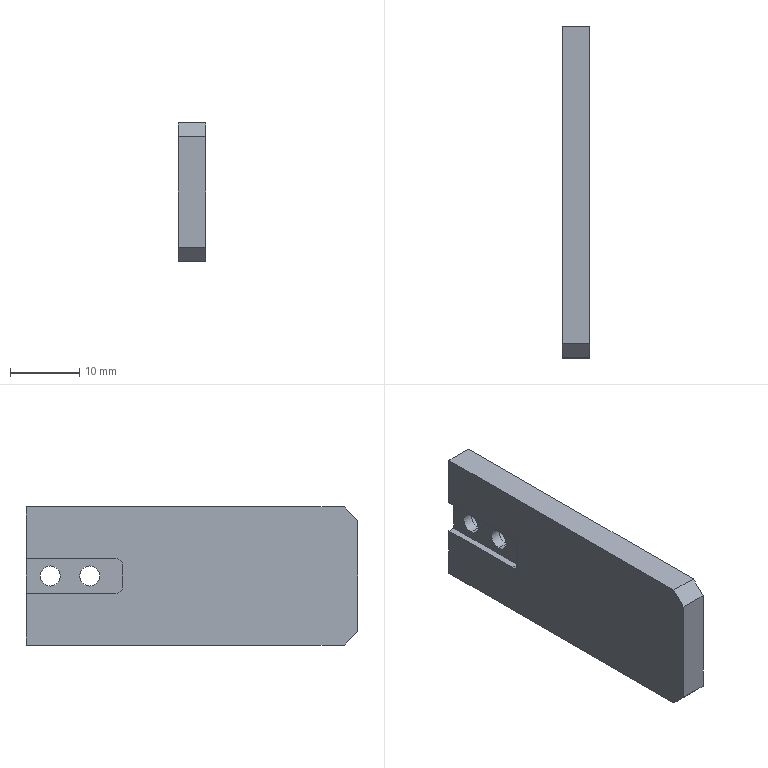Part | STEP file | 0-19 Finger (retainer) | 1 solid | 24 faces | box 4 x 48 x 20 mm | volume 3676 mm3 | plane 14 | cylinder 10 | commonest cylinder face diameters 2.9 x4 5 x4 2 x2